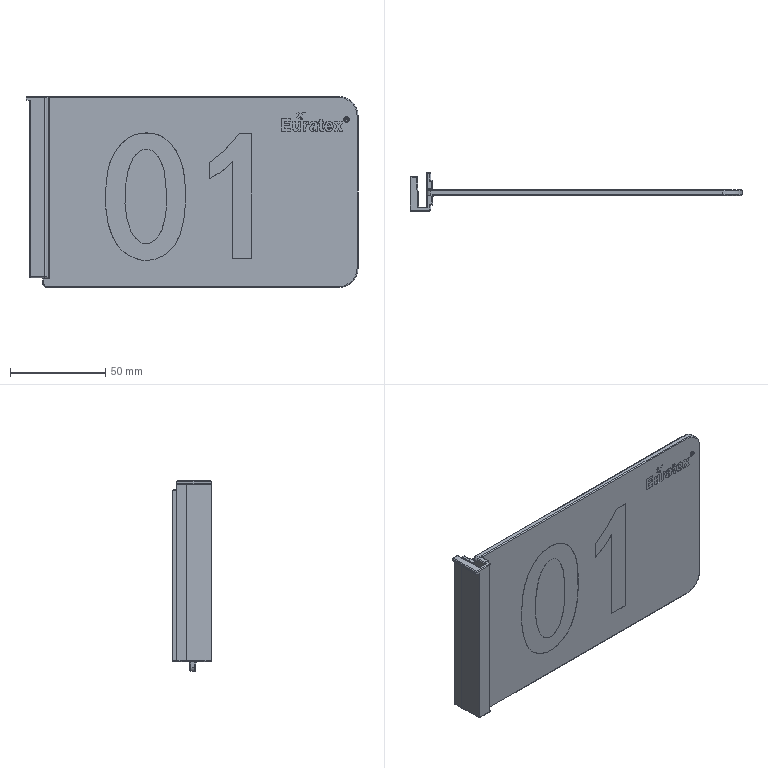Part | STEP file | 51E-01017SL10 | 1 solid | 375 faces | box 173.954 x 20.1 x 100 mm | volume 57654 mm3 | plane 238 | cylinder 75 | spline 46 | torus 16 | commonest cylinder face diameters 1 x46 0.448 x4 0.459 x4 0.83 x4 1.004 x4 2.422 x4